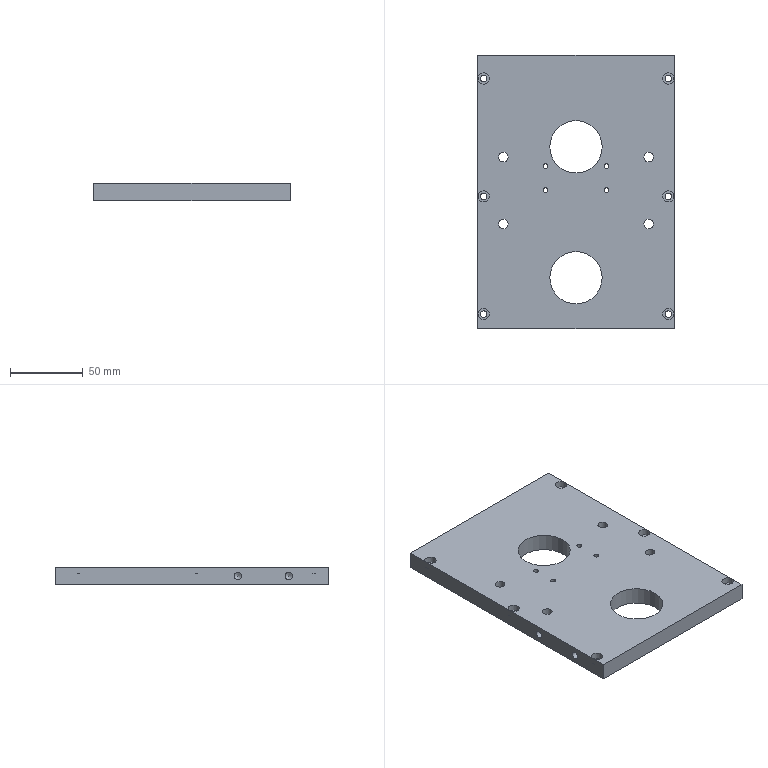Part | NX | 1 solid | 46 faces | box 135 x 188 x 12 mm | volume 273847 mm3 | cylinder 28 | plane 16 | cone 2 | commonest cylinder face diameters 4.5 x6 7.8 x6 3.3 x4 6.6 x4 11 x4 5 x2
STEP:
#1=CARTESIAN_POINT('',(-22.65,66.75,-6.));
#2=VERTEX_POINT('',#1);
#3=CARTESIAN_POINT('',(-21.,66.75,-6.));
#4=DIRECTION('',(0.,0.,-1.));
#5=DIRECTION('',(-1.,0.,0.));
#6=AXIS2_PLACEMENT_3D('',#3,#4,#5);
#7=CIRCLE('',#6,1.65);
#8=EDGE_CURVE('',#2,#2,#7,.T.);
#9=ORIENTED_EDGE('',*,*,#8,.F.);
#10=EDGE_LOOP('',(#9));
#11=FACE_BOUND('',#10,.T.);
#12=CARTESIAN_POINT('',(-22.65,50.25,-6.));
#13=VERTEX_POINT('',#12);
#14=CARTESIAN_POINT('',(-21.,50.25,-6.));
#15=DIRECTION('',(0.,0.,-1.));
#16=DIRECTION('',(-1.,0.,0.));
#17=AXIS2_PLACEMENT_3D('',#14,#15,#16);
#18=CIRCLE('',#17,1.65);
#19=EDGE_CURVE('',#13,#13,#18,.T.);
#20=ORIENTED_EDGE('',*,*,#19,.F.);
#21=EDGE_LOOP('',(#20));
#22=FACE_BOUND('',#21,.T.);
#23=CARTESIAN_POINT('',(19.35,50.25,-6.));
#24=VERTEX_POINT('',#23);
#25=CARTESIAN_POINT('',(21.,50.25,-6.));
#26=DIRECTION('',(0.,0.,-1.));
#27=DIRECTION('',(-1.,0.,0.));
#28=AXIS2_PLACEMENT_3D('',#25,#26,#27);
#29=CIRCLE('',#28,1.65);
#30=EDGE_CURVE('',#24,#24,#29,.T.);
#31=ORIENTED_EDGE('',*,*,#30,.F.);
#32=EDGE_LOOP('',(#31));
#33=FACE_BOUND('',#32,.T.);
#34=CARTESIAN_POINT('',(67.5,-45.,-6.));
#35=VERTEX_POINT('',#34);
#36=CARTESIAN_POINT('',(67.5,143.,-6.));
#37=VERTEX_POINT('',#36);
#38=CARTESIAN_POINT('',(67.5,45.,-6.));
#39=DIRECTION('',(0.,1.,0.));
#40=VECTOR('',#39,1000.);
#41=LINE('',#38,#40);
#42=EDGE_CURVE('',#35,#37,#41,.T.);
#43=ORIENTED_EDGE('',*,*,#42,.F.);
#44=CARTESIAN_POINT('',(-67.5,-45.,-6.));
#45=VERTEX_POINT('',#44);
#46=CARTESIAN_POINT('',(-67.5,-45.,-6.));
#47=DIRECTION('',(1.,0.,0.));
#48=VECTOR('',#47,1000.);
#49=LINE('',#46,#48);
#50=EDGE_CURVE('',#45,#35,#49,.T.);
#51=ORIENTED_EDGE('',*,*,#50,.F.);
#52=CARTESIAN_POINT('',(-67.5,143.,-6.));
#53=VERTEX_POINT('',#52);
#54=CARTESIAN_POINT('',(-67.5,45.,-6.));
#55=DIRECTION('',(0.,-1.,0.));
#56=VECTOR('',#55,1000.);
#57=LINE('',#54,#56);
#58=EDGE_CURVE('',#53,#45,#57,.T.);
#59=ORIENTED_EDGE('',*,*,#58,.F.);
#60=CARTESIAN_POINT('',(-67.5,143.,-6.));
#61=DIRECTION('',(1.,0.,0.));
#62=VECTOR('',#61,1000.);
#63=LINE('',#60,#62);
#64=EDGE_CURVE('',#53,#37,#63,.T.);
#65=ORIENTED_EDGE('',*,*,#64,.T.);
#66=EDGE_LOOP('',(#43,#51,#59,#65));
#67=FACE_BOUND('',#66,.T.);
#68=CARTESIAN_POINT('',(65.75,-35.,-6.));
#69=VERTEX_POINT('',#68);
#70=CARTESIAN_POINT('',(63.5,-35.,-6.));
#71=DIRECTION('',(0.,0.,1.));
#72=DIRECTION('',(1.,0.,0.));
#73=AXIS2_PLACEMENT_3D('',#70,#71,#72);
#74=CIRCLE('',#73,2.25);
#75=EDGE_CURVE('',#69,#69,#74,.T.);
#76=ORIENTED_EDGE('',*,*,#75,.T.);
#77=EDGE_LOOP('',(#76));
#78=FACE_BOUND('',#77,.T.);
#79=CARTESIAN_POINT('',(-61.25,-35.,-6.));
#80=VERTEX_POINT('',#79);
#81=CARTESIAN_POINT('',(-63.5,-35.,-6.));
#82=DIRECTION('',(0.,0.,1.));
#83=DIRECTION('',(1.,0.,0.));
#84=AXIS2_PLACEMENT_3D('',#81,#82,#83);
#85=CIRCLE('',#84,2.25);
#86=EDGE_CURVE('',#80,#80,#85,.T.);
#87=ORIENTED_EDGE('',*,*,#86,.T.);
#88=EDGE_LOOP('',(#87));
#89=FACE_BOUND('',#88,.T.);
#90=CARTESIAN_POINT('',(-61.25,127.,-6.));
#91=VERTEX_POINT('',#90);
#92=CARTESIAN_POINT('',(-63.5,127.,-6.));
#93=DIRECTION('',(0.,0.,1.));
#94=DIRECTION('',(1.,0.,0.));
#95=AXIS2_PLACEMENT_3D('',#92,#93,#94);
#96=CIRCLE('',#95,2.25);
#97=EDGE_CURVE('',#91,#91,#96,.T.);
#98=ORIENTED_EDGE('',*,*,#97,.T.);
#99=EDGE_LOOP('',(#98));
#100=FACE_BOUND('',#99,.T.);
#101=CARTESIAN_POINT('',(-61.25,46.,-6.));
#102=VERTEX_POINT('',#101);
#103=CARTESIAN_POINT('',(-63.5,46.,-6.));
#104=DIRECTION('',(0.,0.,1.));
#105=DIRECTION('',(1.,0.,0.));
#106=AXIS2_PLACEMENT_3D('',#103,#104,#105);
#107=CIRCLE('',#106,2.25);
#108=EDGE_CURVE('',#102,#102,#107,.T.);
#109=ORIENTED_EDGE('',*,*,#108,.T.);
#110=EDGE_LOOP('',(#109));
#111=FACE_BOUND('',#110,.T.);
#112=CARTESIAN_POINT('',(65.75,46.,-6.));
#113=VERTEX_POINT('',#112);
#114=CARTESIAN_POINT('',(63.5,46.,-6.));
#115=DIRECTION('',(0.,0.,1.));
#116=DIRECTION('',(1.,0.,0.));
#117=AXIS2_PLACEMENT_3D('',#114,#115,#116);
#118=CIRCLE('',#117,2.25);
#119=EDGE_CURVE('',#113,#113,#118,.T.);
#120=ORIENTED_EDGE('',*,*,#119,.T.);
#121=EDGE_LOOP('',(#120));
#122=FACE_BOUND('',#121,.T.);
#123=CARTESIAN_POINT('',(65.75,127.,-6.));
#124=VERTEX_POINT('',#123);
#125=CARTESIAN_POINT('',(63.5,127.,-6.));
#126=DIRECTION('',(0.,0.,1.));
#127=DIRECTION('',(1.,0.,0.));
#128=AXIS2_PLACEMENT_3D('',#125,#126,#127);
#129=CIRCLE('',#128,2.25);
#130=EDGE_CURVE('',#124,#124,#129,.T.);
#131=ORIENTED_EDGE('',*,*,#130,.T.);
#132=EDGE_LOOP('',(#131));
#133=FACE_BOUND('',#132,.T.);
#134=CARTESIAN_POINT('',(-55.5,73.,-6.));
#135=VERTEX_POINT('',#134);
#136=CARTESIAN_POINT('',(-50.,73.,-6.));
#137=DIRECTION('',(0.,0.,-1.));
#138=DIRECTION('',(-1.,0.,0.));
#139=AXIS2_PLACEMENT_3D('',#136,#137,#138);
#140=CIRCLE('',#139,5.5);
#141=EDGE_CURVE('',#135,#135,#140,.T.);
#142=ORIENTED_EDGE('',*,*,#141,.F.);
#143=EDGE_LOOP('',(#142));
#144=FACE_BOUND('',#143,.T.);
#145=CARTESIAN_POINT('',(-55.5,27.,-6.));
#146=VERTEX_POINT('',#145);
#147=CARTESIAN_POINT('',(-50.,27.,-6.));
#148=DIRECTION('',(0.,0.,-1.));
#149=DIRECTION('',(-1.,0.,0.));
#150=AXIS2_PLACEMENT_3D('',#147,#148,#149);
#151=CIRCLE('',#150,5.5);
#152=EDGE_CURVE('',#146,#146,#151,.T.);
#153=ORIENTED_EDGE('',*,*,#152,.F.);
#154=EDGE_LOOP('',(#153));
#155=FACE_BOUND('',#154,.T.);
#156=CARTESIAN_POINT('',(44.5,27.,-6.));
#157=VERTEX_POINT('',#156);
#158=CARTESIAN_POINT('',(50.,27.,-6.));
#159=DIRECTION('',(0.,0.,-1.));
#160=DIRECTION('',(-1.,0.,0.));
#161=AXIS2_PLACEMENT_3D('',#158,#159,#160);
#162=CIRCLE('',#161,5.5);
#163=EDGE_CURVE('',#157,#157,#162,.T.);
#164=ORIENTED_EDGE('',*,*,#163,.F.);
#165=EDGE_LOOP('',(#164));
#166=FACE_BOUND('',#165,.T.);
#167=CARTESIAN_POINT('',(44.5,73.,-6.));
#168=VERTEX_POINT('',#167);
#169=CARTESIAN_POINT('',(50.,73.,-6.));
#170=DIRECTION('',(0.,0.,-1.));
#171=DIRECTION('',(-1.,0.,0.));
#172=AXIS2_PLACEMENT_3D('',#169,#170,#171);
#173=CIRCLE('',#172,5.5);
#174=EDGE_CURVE('',#168,#168,#173,.T.);
#175=ORIENTED_EDGE('',*,*,#174,.F.);
#176=EDGE_LOOP('',(#175));
#177=FACE_BOUND('',#176,.T.);
#178=CARTESIAN_POINT('',(18.,80.,-6.));
#179=VERTEX_POINT('',#178);
#180=CARTESIAN_POINT('',(0.,80.,-6.));
#181=DIRECTION('',(0.,0.,1.));
#182=DIRECTION('',(1.,0.,0.));
#183=AXIS2_PLACEMENT_3D('',#180,#181,#182);
#184=CIRCLE('',#183,18.);
#185=EDGE_CURVE('',#179,#179,#184,.T.);
#186=ORIENTED_EDGE('',*,*,#185,.T.);
#187=EDGE_LOOP('',(#186));
#188=FACE_BOUND('',#187,.T.);
#189=CARTESIAN_POINT('',(18.,-10.,-6.));
#190=VERTEX_POINT('',#189);
#191=CARTESIAN_POINT('',(0.,-10.,-6.));
#192=DIRECTION('',(0.,0.,1.));
#193=DIRECTION('',(1.,0.,0.));
#194=AXIS2_PLACEMENT_3D('',#191,#192,#193);
#195=CIRCLE('',#194,18.);
#196=EDGE_CURVE('',#190,#190,#195,.T.);
#197=ORIENTED_EDGE('',*,*,#196,.T.);
#198=EDGE_LOOP('',(#197));
#199=FACE_BOUND('',#198,.T.);
#200=CARTESIAN_POINT('',(19.35,66.75,-6.));
#201=VERTEX_POINT('',#200);
#202=CARTESIAN_POINT('',(21.,66.75,-6.));
#203=DIRECTION('',(0.,0.,-1.));
#204=DIRECTION('',(-1.,0.,0.));
#205=AXIS2_PLACEMENT_3D('',#202,#203,#204);
#206=CIRCLE('',#205,1.65);
#207=EDGE_CURVE('',#201,#201,#206,.T.);
#208=ORIENTED_EDGE('',*,*,#207,.F.);
#209=EDGE_LOOP('',(#208));
#210=FACE_BOUND('',#209,.T.);
#211=CARTESIAN_POINT('',(0.,0.,-6.));
#212=DIRECTION('',(0.,0.,1.));
#213=DIRECTION('',(1.,0.,0.));
#214=AXIS2_PLACEMENT_3D('',#211,#212,#213);
#215=PLANE('',#214);
#216=ADVANCED_FACE('',(#11,#22,#33,#67,#78,#89,#100,#111,#122,#133,#144,#155,#166,#177,#188,#199,#210),#215,.F.);
#217=ORIENTED_EDGE('',*,*,#42,.T.);
#218=CARTESIAN_POINT('',(67.5,143.,6.));
#219=VERTEX_POINT('',#218);
#220=CARTESIAN_POINT('',(67.5,143.,172.82));
#221=DIRECTION('',(0.,0.,-1.));
#222=VECTOR('',#221,1000.);
#223=LINE('',#220,#222);
#224=EDGE_CURVE('',#219,#37,#223,.T.);
#225=ORIENTED_EDGE('',*,*,#224,.F.);
#226=CARTESIAN_POINT('',(67.5,-45.,6.));
#227=VERTEX_POINT('',#226);
#228=CARTESIAN_POINT('',(67.5,45.,6.));
#229=DIRECTION('',(0.,1.,0.));
#230=VECTOR('',#229,1000.);
#231=LINE('',#228,#230);
#232=EDGE_CURVE('',#227,#219,#231,.T.);
#233=ORIENTED_EDGE('',*,*,#232,.F.);
#234=CARTESIAN_POINT('',(67.5,-45.,6.));
#235=DIRECTION('',(0.,0.,-1.));
#236=VECTOR('',#235,1000.);
#237=LINE('',#234,#236);
#238=EDGE_CURVE('',#227,#35,#237,.T.);
#239=ORIENTED_EDGE('',*,*,#238,.T.);
#240=EDGE_LOOP('',(#217,#225,#233,#239));
#241=FACE_BOUND('',#240,.T.);
#242=CARTESIAN_POINT('',(67.5,45.,6.));
#243=DIRECTION('',(-1.,0.,0.));
#244=DIRECTION('',(0.,-1.,0.));
#245=AXIS2_PLACEMENT_3D('',#242,#243,#244);
#246=PLANE('',#245);
#247=ADVANCED_FACE('',(#241),#246,.F.);
#248=CARTESIAN_POINT('',(-67.5,17.5,2.5));
#249=VERTEX_POINT('',#248);
#250=CARTESIAN_POINT('',(-67.5,17.5,0.));
#251=DIRECTION('',(-1.,0.,0.));
#252=DIRECTION('',(0.,0.,1.));
#253=AXIS2_PLACEMENT_3D('',#250,#251,#252);
#254=CIRCLE('',#253,2.5);
#255=EDGE_CURVE('',#249,#249,#254,.T.);
#256=ORIENTED_EDGE('',*,*,#255,.F.);
#257=EDGE_LOOP('',(#256));
#258=FACE_BOUND('',#257,.T.);
#259=CARTESIAN_POINT('',(-67.5,-17.5,2.5));
#260=VERTEX_POINT('',#259);
#261=CARTESIAN_POINT('',(-67.5,-17.5,0.));
#262=DIRECTION('',(-1.,0.,0.));
#263=DIRECTION('',(0.,0.,1.));
#264=AXIS2_PLACEMENT_3D('',#261,#262,#263);
#265=CIRCLE('',#264,2.5);
#266=EDGE_CURVE('',#260,#260,#265,.T.);
#267=ORIENTED_EDGE('',*,*,#266,.F.);
#268=EDGE_LOOP('',(#267));
#269=FACE_BOUND('',#268,.T.);
#270=ORIENTED_EDGE('',*,*,#58,.T.);
#271=CARTESIAN_POINT('',(-67.5,-45.,6.));
#272=VERTEX_POINT('',#271);
#273=CARTESIAN_POINT('',(-67.5,-45.,6.));
#274=DIRECTION('',(0.,0.,-1.));
#275=VECTOR('',#274,1000.);
#276=LINE('',#273,#275);
#277=EDGE_CURVE('',#272,#45,#276,.T.);
#278=ORIENTED_EDGE('',*,*,#277,.F.);
#279=CARTESIAN_POINT('',(-67.5,143.,6.));
#280=VERTEX_POINT('',#279);
#281=CARTESIAN_POINT('',(-67.5,45.,6.));
#282=DIRECTION('',(0.,-1.,0.));
#283=VECTOR('',#282,1000.);
#284=LINE('',#281,#283);
#285=EDGE_CURVE('',#280,#272,#284,.T.);
#286=ORIENTED_EDGE('',*,*,#285,.F.);
#287=CARTESIAN_POINT('',(-67.5,143.,172.82));
#288=DIRECTION('',(0.,0.,-1.));
#289=VECTOR('',#288,1000.);
#290=LINE('',#287,#289);
#291=EDGE_CURVE('',#280,#53,#290,.T.);
#292=ORIENTED_EDGE('',*,*,#291,.T.);
#293=EDGE_LOOP('',(#270,#278,#286,#292));
#294=FACE_BOUND('',#293,.T.);
#295=CARTESIAN_POINT('',(-67.5,45.,6.));
#296=DIRECTION('',(1.,0.,0.));
#297=DIRECTION('',(0.,0.,-1.));
#298=AXIS2_PLACEMENT_3D('',#295,#296,#297);
#299=PLANE('',#298);
#300=ADVANCED_FACE('',(#258,#269,#294),#299,.F.);
#301=ORIENTED_EDGE('',*,*,#50,.T.);
#302=ORIENTED_EDGE('',*,*,#238,.F.);
#303=CARTESIAN_POINT('',(-67.5,-45.,6.));
#304=DIRECTION('',(1.,0.,0.));
#305=VECTOR('',#304,1000.);
#306=LINE('',#303,#305);
#307=EDGE_CURVE('',#272,#227,#306,.T.);
#308=ORIENTED_EDGE('',*,*,#307,.F.);
#309=ORIENTED_EDGE('',*,*,#277,.T.);
#310=EDGE_LOOP('',(#301,#302,#308,#309));
#311=FACE_BOUND('',#310,.T.);
#312=CARTESIAN_POINT('',(-67.5,-45.,6.));
#313=DIRECTION('',(0.,1.,0.));
#314=DIRECTION('',(0.,0.,1.));
#315=AXIS2_PLACEMENT_3D('',#312,#313,#314);
#316=PLANE('',#315);
#317=ADVANCED_FACE('',(#311),#316,.F.);
#318=CARTESIAN_POINT('',(-22.65,66.75,6.));
#319=VERTEX_POINT('',#318);
#320=CARTESIAN_POINT('',(-21.,66.75,6.));
#321=DIRECTION('',(0.,0.,-1.));
#322=DIRECTION('',(-1.,0.,0.));
#323=AXIS2_PLACEMENT_3D('',#320,#321,#322);
#324=CIRCLE('',#323,1.65);
#325=EDGE_CURVE('',#319,#319,#324,.T.);
#326=ORIENTED_EDGE('',*,*,#325,.T.);
#327=EDGE_LOOP('',(#326));
#328=FACE_BOUND('',#327,.T.);
#329=CARTESIAN_POINT('',(-22.65,50.25,6.));
#330=VERTEX_POINT('',#329);
#331=CARTESIAN_POINT('',(-21.,50.25,6.));
#332=DIRECTION('',(0.,0.,-1.));
#333=DIRECTION('',(-1.,0.,0.));
#334=AXIS2_PLACEMENT_3D('',#331,#332,#333);
#335=CIRCLE('',#334,1.65);
#336=EDGE_CURVE('',#330,#330,#335,.T.);
#337=ORIENTED_EDGE('',*,*,#336,.T.);
#338=EDGE_LOOP('',(#337));
#339=FACE_BOUND('',#338,.T.);
#340=CARTESIAN_POINT('',(19.35,50.25,6.));
#341=VERTEX_POINT('',#340);
#342=CARTESIAN_POINT('',(21.,50.25,6.));
#343=DIRECTION('',(0.,0.,-1.));
#344=DIRECTION('',(-1.,0.,0.));
#345=AXIS2_PLACEMENT_3D('',#342,#343,#344);
#346=CIRCLE('',#345,1.65);
#347=EDGE_CURVE('',#341,#341,#346,.T.);
#348=ORIENTED_EDGE('',*,*,#347,.T.);
#349=EDGE_LOOP('',(#348));
#350=FACE_BOUND('',#349,.T.);
#351=CARTESIAN_POINT('',(19.35,66.75,6.));
#352=VERTEX_POINT('',#351);
#353=CARTESIAN_POINT('',(21.,66.75,6.));
#354=DIRECTION('',(0.,0.,-1.));
#355=DIRECTION('',(-1.,0.,0.));
#356=AXIS2_PLACEMENT_3D('',#353,#354,#355);
#357=CIRCLE('',#356,1.65);
#358=EDGE_CURVE('',#352,#352,#357,.T.);
#359=ORIENTED_EDGE('',*,*,#358,.T.);
#360=EDGE_LOOP('',(#359));
#361=FACE_BOUND('',#360,.T.);
#362=CARTESIAN_POINT('',(18.,-10.,6.));
#363=VERTEX_POINT('',#362);
#364=CARTESIAN_POINT('',(0.,-10.,6.));
#365=DIRECTION('',(0.,0.,1.));
#366=DIRECTION('',(1.,0.,0.));
#367=AXIS2_PLACEMENT_3D('',#364,#365,#366);
#368=CIRCLE('',#367,18.);
#369=EDGE_CURVE('',#363,#363,#368,.T.);
#370=ORIENTED_EDGE('',*,*,#369,.F.);
#371=EDGE_LOOP('',(#370));
#372=FACE_BOUND('',#371,.T.);
#373=CARTESIAN_POINT('',(18.,80.,6.));
#374=VERTEX_POINT('',#373);
#375=CARTESIAN_POINT('',(0.,80.,6.));
#376=DIRECTION('',(0.,0.,1.));
#377=DIRECTION('',(1.,0.,0.));
#378=AXIS2_PLACEMENT_3D('',#375,#376,#377);
#379=CIRCLE('',#378,18.);
#380=EDGE_CURVE('',#374,#374,#379,.T.);
#381=ORIENTED_EDGE('',*,*,#380,.F.);
#382=EDGE_LOOP('',(#381));
#383=FACE_BOUND('',#382,.T.);
#384=CARTESIAN_POINT('',(46.7,73.,6.));
#385=VERTEX_POINT('',#384);
#386=CARTESIAN_POINT('',(50.,73.,6.));
#387=DIRECTION('',(0.,0.,-1.));
#388=DIRECTION('',(-1.,0.,0.));
#389=AXIS2_PLACEMENT_3D('',#386,#387,#388);
#390=CIRCLE('',#389,3.3);
#391=EDGE_CURVE('',#385,#385,#390,.T.);
#392=ORIENTED_EDGE('',*,*,#391,.T.);
#393=EDGE_LOOP('',(#392));
#394=FACE_BOUND('',#393,.T.);
#395=CARTESIAN_POINT('',(46.7,27.,6.));
#396=VERTEX_POINT('',#395);
#397=CARTESIAN_POINT('',(50.,27.,6.));
#398=DIRECTION('',(0.,0.,-1.));
#399=DIRECTION('',(-1.,0.,0.));
#400=AXIS2_PLACEMENT_3D('',#397,#398,#399);
#401=CIRCLE('',#400,3.3);
#402=EDGE_CURVE('',#396,#396,#401,.T.);
#403=ORIENTED_EDGE('',*,*,#402,.T.);
#404=EDGE_LOOP('',(#403));
#405=FACE_BOUND('',#404,.T.);
#406=CARTESIAN_POINT('',(-53.3,27.,6.));
#407=VERTEX_POINT('',#406);
#408=CARTESIAN_POINT('',(-50.,27.,6.));
#409=DIRECTION('',(0.,0.,-1.));
#410=DIRECTION('',(-1.,0.,0.));
#411=AXIS2_PLACEMENT_3D('',#408,#409,#410);
#412=CIRCLE('',#411,3.3);
#413=EDGE_CURVE('',#407,#407,#412,.T.);
#414=ORIENTED_EDGE('',*,*,#413,.T.);
#415=EDGE_LOOP('',(#414));
#416=FACE_BOUND('',#415,.T.);
#417=CARTESIAN_POINT('',(-53.3,73.,6.));
#418=VERTEX_POINT('',#417);
#419=CARTESIAN_POINT('',(-50.,73.,6.));
#420=DIRECTION('',(0.,0.,-1.));
#421=DIRECTION('',(-1.,0.,0.));
#422=AXIS2_PLACEMENT_3D('',#419,#420,#421);
#423=CIRCLE('',#422,3.3);
#424=EDGE_CURVE('',#418,#418,#423,.T.);
#425=ORIENTED_EDGE('',*,*,#424,.T.);
#426=EDGE_LOOP('',(#425));
#427=FACE_BOUND('',#426,.T.);
#428=CARTESIAN_POINT('',(67.4,127.,6.));
#429=VERTEX_POINT('',#428);
#430=CARTESIAN_POINT('',(63.5,127.,6.));
#431=DIRECTION('',(0.,0.,1.));
#432=DIRECTION('',(1.,0.,0.));
#433=AXIS2_PLACEMENT_3D('',#430,#431,#432);
#434=CIRCLE('',#433,3.9);
#435=EDGE_CURVE('',#429,#429,#434,.T.);
#436=ORIENTED_EDGE('',*,*,#435,.F.);
#437=EDGE_LOOP('',(#436));
#438=FACE_BOUND('',#437,.T.);
#439=CARTESIAN_POINT('',(67.4,46.,6.));
#440=VERTEX_POINT('',#439);
#441=CARTESIAN_POINT('',(63.5,46.,6.));
#442=DIRECTION('',(0.,0.,1.));
#443=DIRECTION('',(1.,0.,0.));
#444=AXIS2_PLACEMENT_3D('',#441,#442,#443);
#445=CIRCLE('',#444,3.9);
#446=EDGE_CURVE('',#440,#440,#445,.T.);
#447=ORIENTED_EDGE('',*,*,#446,.F.);
#448=EDGE_LOOP('',(#447));
#449=FACE_BOUND('',#448,.T.);
#450=CARTESIAN_POINT('',(-59.6,46.,6.));
#451=VERTEX_POINT('',#450);
#452=CARTESIAN_POINT('',(-63.5,46.,6.));
#453=DIRECTION('',(0.,0.,1.));
#454=DIRECTION('',(1.,0.,0.));
#455=AXIS2_PLACEMENT_3D('',#452,#453,#454);
#456=CIRCLE('',#455,3.9);
#457=EDGE_CURVE('',#451,#451,#456,.T.);
#458=ORIENTED_EDGE('',*,*,#457,.F.);
#459=EDGE_LOOP('',(#458));
#460=FACE_BOUND('',#459,.T.);
#461=CARTESIAN_POINT('',(-59.6,127.,6.));
#462=VERTEX_POINT('',#461);
#463=CARTESIAN_POINT('',(-63.5,127.,6.));
#464=DIRECTION('',(0.,0.,1.));
#465=DIRECTION('',(1.,0.,0.));
#466=AXIS2_PLACEMENT_3D('',#463,#464,#465);
#467=CIRCLE('',#466,3.9);
#468=EDGE_CURVE('',#462,#462,#467,.T.);
#469=ORIENTED_EDGE('',*,*,#468,.F.);
#470=EDGE_LOOP('',(#469));
#471=FACE_BOUND('',#470,.T.);
#472=CARTESIAN_POINT('',(-59.6,-35.,6.));
#473=VERTEX_POINT('',#472);
#474=CARTESIAN_POINT('',(-63.5,-35.,6.));
#475=DIRECTION('',(0.,0.,1.));
#476=DIRECTION('',(1.,0.,0.));
#477=AXIS2_PLACEMENT_3D('',#474,#475,#476);
#478=CIRCLE('',#477,3.9);
#479=EDGE_CURVE('',#473,#473,#478,.T.);
#480=ORIENTED_EDGE('',*,*,#479,.F.);
#481=EDGE_LOOP('',(#480));
#482=FACE_BOUND('',#481,.T.);
#483=CARTESIAN_POINT('',(67.4,-35.,6.));
#484=VERTEX_POINT('',#483);
#485=CARTESIAN_POINT('',(63.5,-35.,6.));
#486=DIRECTION('',(0.,0.,1.));
#487=DIRECTION('',(1.,0.,0.));
#488=AXIS2_PLACEMENT_3D('',#485,#486,#487);
#489=CIRCLE('',#488,3.9);
#490=EDGE_CURVE('',#484,#484,#489,.T.);
#491=ORIENTED_EDGE('',*,*,#490,.F.);
#492=EDGE_LOOP('',(#491));
#493=FACE_BOUND('',#492,.T.);
#494=ORIENTED_EDGE('',*,*,#232,.T.);
#495=CARTESIAN_POINT('',(-67.5,143.,6.));
#496=DIRECTION('',(1.,0.,0.));
#497=VECTOR('',#496,1000.);
#498=LINE('',#495,#497);
#499=EDGE_CURVE('',#280,#219,#498,.T.);
#500=ORIENTED_EDGE('',*,*,#499,.F.);
#501=ORIENTED_EDGE('',*,*,#285,.T.);
#502=ORIENTED_EDGE('',*,*,#307,.T.);
#503=EDGE_LOOP('',(#494,#500,#501,#502));
#504=FACE_BOUND('',#503,.T.);
#505=CARTESIAN_POINT('',(0.,0.,6.));
#506=DIRECTION('',(0.,0.,1.));
#507=DIRECTION('',(1.,0.,0.));
#508=AXIS2_PLACEMENT_3D('',#505,#506,#507);
#509=PLANE('',#508);
#510=ADVANCED_FACE('',(#328,#339,#350,#361,#372,#383,#394,#405,#416,#427,#438,#449,#460,#471,#482,#493,#504),#509,.T.);
#511=ORIENTED_EDGE('',*,*,#291,.F.);
#512=ORIENTED_EDGE('',*,*,#499,.T.);
#513=ORIENTED_EDGE('',*,*,#224,.T.);
#514=ORIENTED_EDGE('',*,*,#64,.F.);
#515=EDGE_LOOP('',(#511,#512,#513,#514));
#516=FACE_BOUND('',#515,.T.);
#517=CARTESIAN_POINT('',(-67.5,143.,172.82));
#518=DIRECTION('',(0.,1.,0.));
#519=DIRECTION('',(0.,0.,1.));
#520=AXIS2_PLACEMENT_3D('',#517,#518,#519);
#521=PLANE('',#520);
#522=ADVANCED_FACE('',(#516),#521,.T.);
#523=ORIENTED_EDGE('',*,*,#75,.F.);
#524=EDGE_LOOP('',(#523));
#525=FACE_BOUND('',#524,.T.);
#526=CARTESIAN_POINT('',(65.75,-35.,1.6));
#527=VERTEX_POINT('',#526);
#528=CARTESIAN_POINT('',(63.5,-35.,1.6));
#529=DIRECTION('',(0.,0.,1.));
#530=DIRECTION('',(1.,0.,0.));
#531=AXIS2_PLACEMENT_3D('',#528,#529,#530);
#532=CIRCLE('',#531,2.25);
#533=EDGE_CURVE('',#527,#527,#532,.T.);
#534=ORIENTED_EDGE('',*,*,#533,.T.);
#535=EDGE_LOOP('',(#534));
#536=FACE_BOUND('',#535,.T.);
#537=CARTESIAN_POINT('',(63.5,-35.,6.));
#538=DIRECTION('',(0.,0.,1.));
#539=DIRECTION('',(1.,0.,0.));
#540=AXIS2_PLACEMENT_3D('',#537,#538,#539);
#541=CYLINDRICAL_SURFACE('',#540,2.25);
#542=ADVANCED_FACE('',(#525,#536),#541,.F.);
#543=ORIENTED_EDGE('',*,*,#533,.F.);
#544=EDGE_LOOP('',(#543));
#545=FACE_BOUND('',#544,.T.);
#546=CARTESIAN_POINT('',(67.4,-35.,1.6));
#547=VERTEX_POINT('',#546);
#548=CARTESIAN_POINT('',(63.5,-35.,1.6));
#549=DIRECTION('',(0.,0.,1.));
#550=DIRECTION('',(1.,0.,0.));
#551=AXIS2_PLACEMENT_3D('',#548,#549,#550);
#552=CIRCLE('',#551,3.9);
#553=EDGE_CURVE('',#547,#547,#552,.T.);
#554=ORIENTED_EDGE('',*,*,#553,.T.);
#555=EDGE_LOOP('',(#554));
#556=FACE_BOUND('',#555,.T.);
#557=CARTESIAN_POINT('',(65.75,-35.,1.6));
#558=DIRECTION('',(0.,0.,-1.));
#559=DIRECTION('',(-1.,0.,0.));
#560=AXIS2_PLACEMENT_3D('',#557,#558,#559);
#561=PLANE('',#560);
#562=ADVANCED_FACE('',(#545,#556),#561,.F.);
#563=ORIENTED_EDGE('',*,*,#553,.F.);
#564=EDGE_LOOP('',(#563));
#565=FACE_BOUND('',#564,.T.);
#566=ORIENTED_EDGE('',*,*,#490,.T.);
#567=EDGE_LOOP('',(#566));
#568=FACE_BOUND('',#567,.T.);
#569=CARTESIAN_POINT('',(63.5,-35.,6.));
#570=DIRECTION('',(0.,0.,1.));
#571=DIRECTION('',(1.,0.,0.));
#572=AXIS2_PLACEMENT_3D('',#569,#570,#571);
#573=CYLINDRICAL_SURFACE('',#572,3.9);
#574=ADVANCED_FACE('',(#565,#568),#573,.F.);
#575=ORIENTED_EDGE('',*,*,#86,.F.);
#576=EDGE_LOOP('',(#575));
#577=FACE_BOUND('',#576,.T.);
#578=CARTESIAN_POINT('',(-61.25,-35.,1.6));
#579=VERTEX_POINT('',#578);
#580=CARTESIAN_POINT('',(-63.5,-35.,1.6));
#581=DIRECTION('',(0.,0.,1.));
#582=DIRECTION('',(1.,0.,0.));
#583=AXIS2_PLACEMENT_3D('',#580,#581,#582);
#584=CIRCLE('',#583,2.25);
#585=EDGE_CURVE('',#579,#579,#584,.T.);
#586=ORIENTED_EDGE('',*,*,#585,.T.);
#587=EDGE_LOOP('',(#586));
#588=FACE_BOUND('',#587,.T.);
#589=CARTESIAN_POINT('',(-63.5,-35.,6.));
#590=DIRECTION('',(0.,0.,1.));
#591=DIRECTION('',(1.,0.,0.));
#592=AXIS2_PLACEMENT_3D('',#589,#590,#591);
#593=CYLINDRICAL_SURFACE('',#592,2.25);
#594=ADVANCED_FACE('',(#577,#588),#593,.F.);
#595=ORIENTED_EDGE('',*,*,#585,.F.);
#596=EDGE_LOOP('',(#595));
#597=FACE_BOUND('',#596,.T.);
#598=CARTESIAN_POINT('',(-59.6,-35.,1.6));
#599=VERTEX_POINT('',#598);
#600=CARTESIAN_POINT('',(-63.5,-35.,1.6));
#601=DIRECTION('',(0.,0.,1.));
#602=DIRECTION('',(1.,0.,0.));
#603=AXIS2_PLACEMENT_3D('',#600,#601,#602);
#604=CIRCLE('',#603,3.9);
#605=EDGE_CURVE('',#599,#599,#604,.T.);
#606=ORIENTED_EDGE('',*,*,#605,.T.);
#607=EDGE_LOOP('',(#606));
#608=FACE_BOUND('',#607,.T.);
#609=CARTESIAN_POINT('',(-61.25,-35.,1.6));
#610=DIRECTION('',(0.,0.,-1.));
#611=DIRECTION('',(-1.,0.,0.));
#612=AXIS2_PLACEMENT_3D('',#609,#610,#611);
#613=PLANE('',#612);
#614=ADVANCED_FACE('',(#597,#608),#613,.F.);
#615=ORIENTED_EDGE('',*,*,#605,.F.);
#616=EDGE_LOOP('',(#615));
#617=FACE_BOUND('',#616,.T.);
#618=ORIENTED_EDGE('',*,*,#479,.T.);
#619=EDGE_LOOP('',(#618));
#620=FACE_BOUND('',#619,.T.);
#621=CARTESIAN_POINT('',(-63.5,-35.,6.));
#622=DIRECTION('',(0.,0.,1.));
#623=DIRECTION('',(1.,0.,0.));
#624=AXIS2_PLACEMENT_3D('',#621,#622,#623);
#625=CYLINDRICAL_SURFACE('',#624,3.9);
#626=ADVANCED_FACE('',(#617,#620),#625,.F.);
#627=ORIENTED_EDGE('',*,*,#97,.F.);
#628=EDGE_LOOP('',(#627));
#629=FACE_BOUND('',#628,.T.);
#630=CARTESIAN_POINT('',(-61.25,127.,1.6));
#631=VERTEX_POINT('',#630);
#632=CARTESIAN_POINT('',(-63.5,127.,1.6));
#633=DIRECTION('',(0.,0.,1.));
#634=DIRECTION('',(1.,0.,0.));
#635=AXIS2_PLACEMENT_3D('',#632,#633,#634);
#636=CIRCLE('',#635,2.25);
#637=EDGE_CURVE('',#631,#631,#636,.T.);
#638=ORIENTED_EDGE('',*,*,#637,.T.);
#639=EDGE_LOOP('',(#638));
#640=FACE_BOUND('',#639,.T.);
#641=CARTESIAN_POINT('',(-63.5,127.,6.));
#642=DIRECTION('',(0.,0.,1.));
#643=DIRECTION('',(1.,0.,0.));
#644=AXIS2_PLACEMENT_3D('',#641,#642,#643);
#645=CYLINDRICAL_SURFACE('',#644,2.25);
#646=ADVANCED_FACE('',(#629,#640),#645,.F.);
#647=ORIENTED_EDGE('',*,*,#637,.F.);
#648=EDGE_LOOP('',(#647));
#649=FACE_BOUND('',#648,.T.);
#650=CARTESIAN_POINT('',(-59.6,127.,1.6));
#651=VERTEX_POINT('',#650);
#652=CARTESIAN_POINT('',(-63.5,127.,1.6));
#653=DIRECTION('',(0.,0.,1.));
#654=DIRECTION('',(1.,0.,0.));
#655=AXIS2_PLACEMENT_3D('',#652,#653,#654);
#656=CIRCLE('',#655,3.9);
#657=EDGE_CURVE('',#651,#651,#656,.T.);
#658=ORIENTED_EDGE('',*,*,#657,.T.);
#659=EDGE_LOOP('',(#658));
#660=FACE_BOUND('',#659,.T.);
#661=CARTESIAN_POINT('',(-61.25,127.,1.6));
#662=DIRECTION('',(0.,0.,-1.));
#663=DIRECTION('',(-1.,0.,0.));
#664=AXIS2_PLACEMENT_3D('',#661,#662,#663);
#665=PLANE('',#664);
#666=ADVANCED_FACE('',(#649,#660),#665,.F.);
#667=ORIENTED_EDGE('',*,*,#657,.F.);
#668=EDGE_LOOP('',(#667));
#669=FACE_BOUND('',#668,.T.);
#670=ORIENTED_EDGE('',*,*,#468,.T.);
#671=EDGE_LOOP('',(#670));
#672=FACE_BOUND('',#671,.T.);
#673=CARTESIAN_POINT('',(-63.5,127.,6.));
#674=DIRECTION('',(0.,0.,1.));
#675=DIRECTION('',(1.,0.,0.));
#676=AXIS2_PLACEMENT_3D('',#673,#674,#675);
#677=CYLINDRICAL_SURFACE('',#676,3.9);
#678=ADVANCED_FACE('',(#669,#672),#677,.F.);
#679=ORIENTED_EDGE('',*,*,#108,.F.);
#680=EDGE_LOOP('',(#679));
#681=FACE_BOUND('',#680,.T.);
#682=CARTESIAN_POINT('',(-61.25,46.,1.6));
#683=VERTEX_POINT('',#682);
#684=CARTESIAN_POINT('',(-63.5,46.,1.6));
#685=DIRECTION('',(0.,0.,1.));
#686=DIRECTION('',(1.,0.,0.));
#687=AXIS2_PLACEMENT_3D('',#684,#685,#686);
#688=CIRCLE('',#687,2.25);
#689=EDGE_CURVE('',#683,#683,#688,.T.);
#690=ORIENTED_EDGE('',*,*,#689,.T.);
#691=EDGE_LOOP('',(#690));
#692=FACE_BOUND('',#691,.T.);
#693=CARTESIAN_POINT('',(-63.5,46.,6.));
#694=DIRECTION('',(0.,0.,1.));
#695=DIRECTION('',(1.,0.,0.));
#696=AXIS2_PLACEMENT_3D('',#693,#694,#695);
#697=CYLINDRICAL_SURFACE('',#696,2.25);
#698=ADVANCED_FACE('',(#681,#692),#697,.F.);
#699=ORIENTED_EDGE('',*,*,#689,.F.);
#700=EDGE_LOOP('',(#699));
#701=FACE_BOUND('',#700,.T.);
#702=CARTESIAN_POINT('',(-59.6,46.,1.6));
#703=VERTEX_POINT('',#702);
#704=CARTESIAN_POINT('',(-63.5,46.,1.6));
#705=DIRECTION('',(0.,0.,1.));
#706=DIRECTION('',(1.,0.,0.));
#707=AXIS2_PLACEMENT_3D('',#704,#705,#706);
#708=CIRCLE('',#707,3.9);
#709=EDGE_CURVE('',#703,#703,#708,.T.);
#710=ORIENTED_EDGE('',*,*,#709,.T.);
#711=EDGE_LOOP('',(#710));
#712=FACE_BOUND('',#711,.T.);
#713=CARTESIAN_POINT('',(-61.25,46.,1.6));
#714=DIRECTION('',(0.,0.,-1.));
#715=DIRECTION('',(-1.,0.,0.));
#716=AXIS2_PLACEMENT_3D('',#713,#714,#715);
#717=PLANE('',#716);
#718=ADVANCED_FACE('',(#701,#712),#717,.F.);
#719=ORIENTED_EDGE('',*,*,#709,.F.);
#720=EDGE_LOOP('',(#719));
#721=FACE_BOUND('',#720,.T.);
#722=ORIENTED_EDGE('',*,*,#457,.T.);
#723=EDGE_LOOP('',(#722));
#724=FACE_BOUND('',#723,.T.);
#725=CARTESIAN_POINT('',(-63.5,46.,6.));
#726=DIRECTION('',(0.,0.,1.));
#727=DIRECTION('',(1.,0.,0.));
#728=AXIS2_PLACEMENT_3D('',#725,#726,#727);
#729=CYLINDRICAL_SURFACE('',#728,3.9);
#730=ADVANCED_FACE('',(#721,#724),#729,.F.);
#731=ORIENTED_EDGE('',*,*,#119,.F.);
#732=EDGE_LOOP('',(#731));
#733=FACE_BOUND('',#732,.T.);
#734=CARTESIAN_POINT('',(65.75,46.,1.6));
#735=VERTEX_POINT('',#734);
#736=CARTESIAN_POINT('',(63.5,46.,1.6));
#737=DIRECTION('',(0.,0.,1.));
#738=DIRECTION('',(1.,0.,0.));
#739=AXIS2_PLACEMENT_3D('',#736,#737,#738);
#740=CIRCLE('',#739,2.25);
#741=EDGE_CURVE('',#735,#735,#740,.T.);
#742=ORIENTED_EDGE('',*,*,#741,.T.);
#743=EDGE_LOOP('',(#742));
#744=FACE_BOUND('',#743,.T.);
#745=CARTESIAN_POINT('',(63.5,46.,6.));
#746=DIRECTION('',(0.,0.,1.));
#747=DIRECTION('',(1.,0.,0.));
#748=AXIS2_PLACEMENT_3D('',#745,#746,#747);
#749=CYLINDRICAL_SURFACE('',#748,2.25);
#750=ADVANCED_FACE('',(#733,#744),#749,.F.);
#751=ORIENTED_EDGE('',*,*,#741,.F.);
#752=EDGE_LOOP('',(#751));
#753=FACE_BOUND('',#752,.T.);
#754=CARTESIAN_POINT('',(67.4,46.,1.6));
#755=VERTEX_POINT('',#754);
#756=CARTESIAN_POINT('',(63.5,46.,1.6));
#757=DIRECTION('',(0.,0.,1.));
#758=DIRECTION('',(1.,0.,0.));
#759=AXIS2_PLACEMENT_3D('',#756,#757,#758);
#760=CIRCLE('',#759,3.9);
#761=EDGE_CURVE('',#755,#755,#760,.T.);
#762=ORIENTED_EDGE('',*,*,#761,.T.);
#763=EDGE_LOOP('',(#762));
#764=FACE_BOUND('',#763,.T.);
#765=CARTESIAN_POINT('',(65.75,46.,1.6));
#766=DIRECTION('',(0.,0.,-1.));
#767=DIRECTION('',(-1.,0.,0.));
#768=AXIS2_PLACEMENT_3D('',#765,#766,#767);
#769=PLANE('',#768);
#770=ADVANCED_FACE('',(#753,#764),#769,.F.);
#771=ORIENTED_EDGE('',*,*,#761,.F.);
#772=EDGE_LOOP('',(#771));
#773=FACE_BOUND('',#772,.T.);
#774=ORIENTED_EDGE('',*,*,#446,.T.);
#775=EDGE_LOOP('',(#774));
#776=FACE_BOUND('',#775,.T.);
#777=CARTESIAN_POINT('',(63.5,46.,6.));
#778=DIRECTION('',(0.,0.,1.));
#779=DIRECTION('',(1.,0.,0.));
#780=AXIS2_PLACEMENT_3D('',#777,#778,#779);
#781=CYLINDRICAL_SURFACE('',#780,3.9);
#782=ADVANCED_FACE('',(#773,#776),#781,.F.);
#783=ORIENTED_EDGE('',*,*,#130,.F.);
#784=EDGE_LOOP('',(#783));
#785=FACE_BOUND('',#784,.T.);
#786=CARTESIAN_POINT('',(65.75,127.,1.6));
#787=VERTEX_POINT('',#786);
#788=CARTESIAN_POINT('',(63.5,127.,1.6));
#789=DIRECTION('',(0.,0.,1.));
#790=DIRECTION('',(1.,0.,0.));
#791=AXIS2_PLACEMENT_3D('',#788,#789,#790);
#792=CIRCLE('',#791,2.25);
#793=EDGE_CURVE('',#787,#787,#792,.T.);
#794=ORIENTED_EDGE('',*,*,#793,.T.);
#795=EDGE_LOOP('',(#794));
#796=FACE_BOUND('',#795,.T.);
#797=CARTESIAN_POINT('',(63.5,127.,6.));
#798=DIRECTION('',(0.,0.,1.));
#799=DIRECTION('',(1.,0.,0.));
#800=AXIS2_PLACEMENT_3D('',#797,#798,#799);
#801=CYLINDRICAL_SURFACE('',#800,2.25);
#802=ADVANCED_FACE('',(#785,#796),#801,.F.);
#803=ORIENTED_EDGE('',*,*,#793,.F.);
#804=EDGE_LOOP('',(#803));
#805=FACE_BOUND('',#804,.T.);
#806=CARTESIAN_POINT('',(67.4,127.,1.6));
#807=VERTEX_POINT('',#806);
#808=CARTESIAN_POINT('',(63.5,127.,1.6));
#809=DIRECTION('',(0.,0.,1.));
#810=DIRECTION('',(1.,0.,0.));
#811=AXIS2_PLACEMENT_3D('',#808,#809,#810);
#812=CIRCLE('',#811,3.9);
#813=EDGE_CURVE('',#807,#807,#812,.T.);
#814=ORIENTED_EDGE('',*,*,#813,.T.);
#815=EDGE_LOOP('',(#814));
#816=FACE_BOUND('',#815,.T.);
#817=CARTESIAN_POINT('',(65.75,127.,1.6));
#818=DIRECTION('',(0.,0.,-1.));
#819=DIRECTION('',(-1.,0.,0.));
#820=AXIS2_PLACEMENT_3D('',#817,#818,#819);
#821=PLANE('',#820);
#822=ADVANCED_FACE('',(#805,#816),#821,.F.);
#823=ORIENTED_EDGE('',*,*,#813,.F.);
#824=EDGE_LOOP('',(#823));
#825=FACE_BOUND('',#824,.T.);
#826=ORIENTED_EDGE('',*,*,#435,.T.);
#827=EDGE_LOOP('',(#826));
#828=FACE_BOUND('',#827,.T.);
#829=CARTESIAN_POINT('',(63.5,127.,6.));
#830=DIRECTION('',(0.,0.,1.));
#831=DIRECTION('',(1.,0.,0.));
#832=AXIS2_PLACEMENT_3D('',#829,#830,#831);
#833=CYLINDRICAL_SURFACE('',#832,3.9);
#834=ADVANCED_FACE('',(#825,#828),#833,.F.);
#835=ORIENTED_EDGE('',*,*,#424,.F.);
#836=EDGE_LOOP('',(#835));
#837=FACE_BOUND('',#836,.T.);
#838=CARTESIAN_POINT('',(-53.3,73.,0.4));
#839=VERTEX_POINT('',#838);
#840=CARTESIAN_POINT('',(-50.,73.,0.4));
#841=DIRECTION('',(0.,0.,-1.));
#842=DIRECTION('',(-1.,0.,0.));
#843=AXIS2_PLACEMENT_3D('',#840,#841,#842);
#844=CIRCLE('',#843,3.3);
#845=EDGE_CURVE('',#839,#839,#844,.T.);
#846=ORIENTED_EDGE('',*,*,#845,.T.);
#847=EDGE_LOOP('',(#846));
#848=FACE_BOUND('',#847,.T.);
#849=CARTESIAN_POINT('',(-50.,73.,-6.));
#850=DIRECTION('',(0.,0.,-1.));
#851=DIRECTION('',(-1.,0.,0.));
#852=AXIS2_PLACEMENT_3D('',#849,#850,#851);
#853=CYLINDRICAL_SURFACE('',#852,3.3);
#854=ADVANCED_FACE('',(#837,#848),#853,.F.);
#855=ORIENTED_EDGE('',*,*,#845,.F.);
#856=EDGE_LOOP('',(#855));
#857=FACE_BOUND('',#856,.T.);
#858=CARTESIAN_POINT('',(-55.5,73.,0.4));
#859=VERTEX_POINT('',#858);
#860=CARTESIAN_POINT('',(-50.,73.,0.4));
#861=DIRECTION('',(0.,0.,-1.));
#862=DIRECTION('',(-1.,0.,0.));
#863=AXIS2_PLACEMENT_3D('',#860,#861,#862);
#864=CIRCLE('',#863,5.5);
#865=EDGE_CURVE('',#859,#859,#864,.T.);
#866=ORIENTED_EDGE('',*,*,#865,.T.);
#867=EDGE_LOOP('',(#866));
#868=FACE_BOUND('',#867,.T.);
#869=CARTESIAN_POINT('',(-46.7,73.,0.4));
#870=DIRECTION('',(0.,0.,1.));
#871=DIRECTION('',(1.,0.,0.));
#872=AXIS2_PLACEMENT_3D('',#869,#870,#871);
#873=PLANE('',#872);
#874=ADVANCED_FACE('',(#857,#868),#873,.F.);
#875=ORIENTED_EDGE('',*,*,#865,.F.);
#876=EDGE_LOOP('',(#875));
#877=FACE_BOUND('',#876,.T.);
#878=ORIENTED_EDGE('',*,*,#141,.T.);
#879=EDGE_LOOP('',(#878));
#880=FACE_BOUND('',#879,.T.);
#881=CARTESIAN_POINT('',(-50.,73.,-6.));
#882=DIRECTION('',(0.,0.,-1.));
#883=DIRECTION('',(-1.,0.,0.));
#884=AXIS2_PLACEMENT_3D('',#881,#882,#883);
#885=CYLINDRICAL_SURFACE('',#884,5.5);
#886=ADVANCED_FACE('',(#877,#880),#885,.F.);
#887=ORIENTED_EDGE('',*,*,#413,.F.);
#888=EDGE_LOOP('',(#887));
#889=FACE_BOUND('',#888,.T.);
#890=CARTESIAN_POINT('',(-53.3,27.,0.4));
#891=VERTEX_POINT('',#890);
#892=CARTESIAN_POINT('',(-50.,27.,0.4));
#893=DIRECTION('',(0.,0.,-1.));
#894=DIRECTION('',(-1.,0.,0.));
#895=AXIS2_PLACEMENT_3D('',#892,#893,#894);
#896=CIRCLE('',#895,3.3);
#897=EDGE_CURVE('',#891,#891,#896,.T.);
#898=ORIENTED_EDGE('',*,*,#897,.T.);
#899=EDGE_LOOP('',(#898));
#900=FACE_BOUND('',#899,.T.);
#901=CARTESIAN_POINT('',(-50.,27.,-6.));
#902=DIRECTION('',(0.,0.,-1.));
#903=DIRECTION('',(-1.,0.,0.));
#904=AXIS2_PLACEMENT_3D('',#901,#902,#903);
#905=CYLINDRICAL_SURFACE('',#904,3.3);
#906=ADVANCED_FACE('',(#889,#900),#905,.F.);
#907=ORIENTED_EDGE('',*,*,#897,.F.);
#908=EDGE_LOOP('',(#907));
#909=FACE_BOUND('',#908,.T.);
#910=CARTESIAN_POINT('',(-55.5,27.,0.4));
#911=VERTEX_POINT('',#910);
#912=CARTESIAN_POINT('',(-50.,27.,0.4));
#913=DIRECTION('',(0.,0.,-1.));
#914=DIRECTION('',(-1.,0.,0.));
#915=AXIS2_PLACEMENT_3D('',#912,#913,#914);
#916=CIRCLE('',#915,5.5);
#917=EDGE_CURVE('',#911,#911,#916,.T.);
#918=ORIENTED_EDGE('',*,*,#917,.T.);
#919=EDGE_LOOP('',(#918));
#920=FACE_BOUND('',#919,.T.);
#921=CARTESIAN_POINT('',(-46.7,27.,0.4));
#922=DIRECTION('',(0.,0.,1.));
#923=DIRECTION('',(1.,0.,0.));
#924=AXIS2_PLACEMENT_3D('',#921,#922,#923);
#925=PLANE('',#924);
#926=ADVANCED_FACE('',(#909,#920),#925,.F.);
#927=ORIENTED_EDGE('',*,*,#917,.F.);
#928=EDGE_LOOP('',(#927));
#929=FACE_BOUND('',#928,.T.);
#930=ORIENTED_EDGE('',*,*,#152,.T.);
#931=EDGE_LOOP('',(#930));
#932=FACE_BOUND('',#931,.T.);
#933=CARTESIAN_POINT('',(-50.,27.,-6.));
#934=DIRECTION('',(0.,0.,-1.));
#935=DIRECTION('',(-1.,0.,0.));
#936=AXIS2_PLACEMENT_3D('',#933,#934,#935);
#937=CYLINDRICAL_SURFACE('',#936,5.5);
#938=ADVANCED_FACE('',(#929,#932),#937,.F.);
#939=ORIENTED_EDGE('',*,*,#402,.F.);
#940=EDGE_LOOP('',(#939));
#941=FACE_BOUND('',#940,.T.);
#942=CARTESIAN_POINT('',(46.7,27.,0.4));
#943=VERTEX_POINT('',#942);
#944=CARTESIAN_POINT('',(50.,27.,0.4));
#945=DIRECTION('',(0.,0.,-1.));
#946=DIRECTION('',(-1.,0.,0.));
#947=AXIS2_PLACEMENT_3D('',#944,#945,#946);
#948=CIRCLE('',#947,3.3);
#949=EDGE_CURVE('',#943,#943,#948,.T.);
#950=ORIENTED_EDGE('',*,*,#949,.T.);
#951=EDGE_LOOP('',(#950));
#952=FACE_BOUND('',#951,.T.);
#953=CARTESIAN_POINT('',(50.,27.,-6.));
#954=DIRECTION('',(0.,0.,-1.));
#955=DIRECTION('',(-1.,0.,0.));
#956=AXIS2_PLACEMENT_3D('',#953,#954,#955);
#957=CYLINDRICAL_SURFACE('',#956,3.3);
#958=ADVANCED_FACE('',(#941,#952),#957,.F.);
#959=ORIENTED_EDGE('',*,*,#949,.F.);
#960=EDGE_LOOP('',(#959));
#961=FACE_BOUND('',#960,.T.);
#962=CARTESIAN_POINT('',(44.5,27.,0.4));
#963=VERTEX_POINT('',#962);
#964=CARTESIAN_POINT('',(50.,27.,0.4));
#965=DIRECTION('',(0.,0.,-1.));
#966=DIRECTION('',(-1.,0.,0.));
#967=AXIS2_PLACEMENT_3D('',#964,#965,#966);
#968=CIRCLE('',#967,5.5);
#969=EDGE_CURVE('',#963,#963,#968,.T.);
#970=ORIENTED_EDGE('',*,*,#969,.T.);
#971=EDGE_LOOP('',(#970));
#972=FACE_BOUND('',#971,.T.);
#973=CARTESIAN_POINT('',(53.3,27.,0.4));
#974=DIRECTION('',(0.,0.,1.));
#975=DIRECTION('',(1.,0.,0.));
#976=AXIS2_PLACEMENT_3D('',#973,#974,#975);
#977=PLANE('',#976);
#978=ADVANCED_FACE('',(#961,#972),#977,.F.);
#979=ORIENTED_EDGE('',*,*,#969,.F.);
#980=EDGE_LOOP('',(#979));
#981=FACE_BOUND('',#980,.T.);
#982=ORIENTED_EDGE('',*,*,#163,.T.);
#983=EDGE_LOOP('',(#982));
#984=FACE_BOUND('',#983,.T.);
#985=CARTESIAN_POINT('',(50.,27.,-6.));
#986=DIRECTION('',(0.,0.,-1.));
#987=DIRECTION('',(-1.,0.,0.));
#988=AXIS2_PLACEMENT_3D('',#985,#986,#987);
#989=CYLINDRICAL_SURFACE('',#988,5.5);
#990=ADVANCED_FACE('',(#981,#984),#989,.F.);
#991=ORIENTED_EDGE('',*,*,#391,.F.);
#992=EDGE_LOOP('',(#991));
#993=FACE_BOUND('',#992,.T.);
#994=CARTESIAN_POINT('',(46.7,73.,0.4));
#995=VERTEX_POINT('',#994);
#996=CARTESIAN_POINT('',(50.,73.,0.4));
#997=DIRECTION('',(0.,0.,-1.));
#998=DIRECTION('',(-1.,0.,0.));
#999=AXIS2_PLACEMENT_3D('',#996,#997,#998);
#1000=CIRCLE('',#999,3.3);
#1001=EDGE_CURVE('',#995,#995,#1000,.T.);
#1002=ORIENTED_EDGE('',*,*,#1001,.T.);
#1003=EDGE_LOOP('',(#1002));
#1004=FACE_BOUND('',#1003,.T.);
#1005=CARTESIAN_POINT('',(50.,73.,-6.));
#1006=DIRECTION('',(0.,0.,-1.));
#1007=DIRECTION('',(-1.,0.,0.));
#1008=AXIS2_PLACEMENT_3D('',#1005,#1006,#1007);
#1009=CYLINDRICAL_SURFACE('',#1008,3.3);
#1010=ADVANCED_FACE('',(#993,#1004),#1009,.F.);
#1011=ORIENTED_EDGE('',*,*,#1001,.F.);
#1012=EDGE_LOOP('',(#1011));
#1013=FACE_BOUND('',#1012,.T.);
#1014=CARTESIAN_POINT('',(44.5,73.,0.4));
#1015=VERTEX_POINT('',#1014);
#1016=CARTESIAN_POINT('',(50.,73.,0.4));
#1017=DIRECTION('',(0.,0.,-1.));
#1018=DIRECTION('',(-1.,0.,0.));
#1019=AXIS2_PLACEMENT_3D('',#1016,#1017,#1018);
#1020=CIRCLE('',#1019,5.5);
#1021=EDGE_CURVE('',#1015,#1015,#1020,.T.);
#1022=ORIENTED_EDGE('',*,*,#1021,.T.);
#1023=EDGE_LOOP('',(#1022));
#1024=FACE_BOUND('',#1023,.T.);
#1025=CARTESIAN_POINT('',(53.3,73.,0.4));
#1026=DIRECTION('',(0.,0.,1.));
#1027=DIRECTION('',(1.,0.,0.));
#1028=AXIS2_PLACEMENT_3D('',#1025,#1026,#1027);
#1029=PLANE('',#1028);
#1030=ADVANCED_FACE('',(#1013,#1024),#1029,.F.);
#1031=ORIENTED_EDGE('',*,*,#1021,.F.);
#1032=EDGE_LOOP('',(#1031));
#1033=FACE_BOUND('',#1032,.T.);
#1034=ORIENTED_EDGE('',*,*,#174,.T.);
#1035=EDGE_LOOP('',(#1034));
#1036=FACE_BOUND('',#1035,.T.);
#1037=CARTESIAN_POINT('',(50.,73.,-6.));
#1038=DIRECTION('',(0.,0.,-1.));
#1039=DIRECTION('',(-1.,0.,0.));
#1040=AXIS2_PLACEMENT_3D('',#1037,#1038,#1039);
#1041=CYLINDRICAL_SURFACE('',#1040,5.5);
#1042=ADVANCED_FACE('',(#1033,#1036),#1041,.F.);
#1043=ORIENTED_EDGE('',*,*,#185,.F.);
#1044=EDGE_LOOP('',(#1043));
#1045=FACE_BOUND('',#1044,.T.);
#1046=ORIENTED_EDGE('',*,*,#380,.T.);
#1047=EDGE_LOOP('',(#1046));
#1048=FACE_BOUND('',#1047,.T.);
#1049=CARTESIAN_POINT('',(0.,80.,-6.));
#1050=DIRECTION('',(0.,0.,1.));
#1051=DIRECTION('',(1.,0.,0.));
#1052=AXIS2_PLACEMENT_3D('',#1049,#1050,#1051);
#1053=CYLINDRICAL_SURFACE('',#1052,18.);
#1054=ADVANCED_FACE('',(#1045,#1048),#1053,.F.);
#1055=ORIENTED_EDGE('',*,*,#196,.F.);
#1056=EDGE_LOOP('',(#1055));
#1057=FACE_BOUND('',#1056,.T.);
#1058=ORIENTED_EDGE('',*,*,#369,.T.);
#1059=EDGE_LOOP('',(#1058));
#1060=FACE_BOUND('',#1059,.T.);
#1061=CARTESIAN_POINT('',(0.,-10.,-6.));
#1062=DIRECTION('',(0.,0.,1.));
#1063=DIRECTION('',(1.,0.,0.));
#1064=AXIS2_PLACEMENT_3D('',#1061,#1062,#1063);
#1065=CYLINDRICAL_SURFACE('',#1064,18.);
#1066=ADVANCED_FACE('',(#1057,#1060),#1065,.F.);
#1067=CARTESIAN_POINT('',(-48.998,-17.5,0.));
#1068=VERTEX_POINT('',#1067);
#1069=VERTEX_LOOP('',#1068);
#1070=FACE_BOUND('',#1069,.T.);
#1071=CARTESIAN_POINT('',(-50.5,-17.5,2.5));
#1072=VERTEX_POINT('',#1071);
#1073=CARTESIAN_POINT('',(-50.5,-17.5,0.));
#1074=DIRECTION('',(-1.,0.,0.));
#1075=DIRECTION('',(0.,0.,1.));
#1076=AXIS2_PLACEMENT_3D('',#1073,#1074,#1075);
#1077=CIRCLE('',#1076,2.5);
#1078=EDGE_CURVE('',#1072,#1072,#1077,.T.);
#1079=ORIENTED_EDGE('',*,*,#1078,.T.);
#1080=EDGE_LOOP('',(#1079));
#1081=FACE_BOUND('',#1080,.T.);
#1082=CARTESIAN_POINT('',(-50.5,-17.5,0.));
#1083=DIRECTION('',(-1.,0.,0.));
#1084=DIRECTION('',(0.,0.,1.));
#1085=AXIS2_PLACEMENT_3D('',#1082,#1083,#1084);
#1086=CONICAL_SURFACE('',#1085,2.5,1.03);
#1087=ADVANCED_FACE('',(#1070,#1081),#1086,.F.);
#1088=ORIENTED_EDGE('',*,*,#1078,.F.);
#1089=EDGE_LOOP('',(#1088));
#1090=FACE_BOUND('',#1089,.T.);
#1091=ORIENTED_EDGE('',*,*,#266,.T.);
#1092=EDGE_LOOP('',(#1091));
#1093=FACE_BOUND('',#1092,.T.);
#1094=CARTESIAN_POINT('',(-67.5,-17.5,0.));
#1095=DIRECTION('',(-1.,0.,0.));
#1096=DIRECTION('',(0.,0.,1.));
#1097=AXIS2_PLACEMENT_3D('',#1094,#1095,#1096);
#1098=CYLINDRICAL_SURFACE('',#1097,2.5);
#1099=ADVANCED_FACE('',(#1090,#1093),#1098,.F.);
#1100=CARTESIAN_POINT('',(-48.998,17.5,0.));
#1101=VERTEX_POINT('',#1100);
#1102=VERTEX_LOOP('',#1101);
#1103=FACE_BOUND('',#1102,.T.);
#1104=CARTESIAN_POINT('',(-50.5,17.5,2.5));
#1105=VERTEX_POINT('',#1104);
#1106=CARTESIAN_POINT('',(-50.5,17.5,0.));
#1107=DIRECTION('',(-1.,0.,0.));
#1108=DIRECTION('',(0.,0.,1.));
#1109=AXIS2_PLACEMENT_3D('',#1106,#1107,#1108);
#1110=CIRCLE('',#1109,2.5);
#1111=EDGE_CURVE('',#1105,#1105,#1110,.T.);
#1112=ORIENTED_EDGE('',*,*,#1111,.T.);
#1113=EDGE_LOOP('',(#1112));
#1114=FACE_BOUND('',#1113,.T.);
#1115=CARTESIAN_POINT('',(-50.5,17.5,0.));
#1116=DIRECTION('',(-1.,0.,0.));
#1117=DIRECTION('',(0.,0.,1.));
#1118=AXIS2_PLACEMENT_3D('',#1115,#1116,#1117);
#1119=CONICAL_SURFACE('',#1118,2.5,1.03);
#1120=ADVANCED_FACE('',(#1103,#1114),#1119,.F.);
#1121=ORIENTED_EDGE('',*,*,#1111,.F.);
#1122=EDGE_LOOP('',(#1121));
#1123=FACE_BOUND('',#1122,.T.);
#1124=ORIENTED_EDGE('',*,*,#255,.T.);
#1125=EDGE_LOOP('',(#1124));
#1126=FACE_BOUND('',#1125,.T.);
#1127=CARTESIAN_POINT('',(-67.5,17.5,0.));
#1128=DIRECTION('',(-1.,0.,0.));
#1129=DIRECTION('',(0.,0.,1.));
#1130=AXIS2_PLACEMENT_3D('',#1127,#1128,#1129);
#1131=CYLINDRICAL_SURFACE('',#1130,2.5);
#1132=ADVANCED_FACE('',(#1123,#1126),#1131,.F.);
#1133=ORIENTED_EDGE('',*,*,#358,.F.);
#1134=EDGE_LOOP('',(#1133));
#1135=FACE_BOUND('',#1134,.T.);
#1136=ORIENTED_EDGE('',*,*,#207,.T.);
#1137=EDGE_LOOP('',(#1136));
#1138=FACE_BOUND('',#1137,.T.);
#1139=CARTESIAN_POINT('',(21.,66.75,-6.));
#1140=DIRECTION('',(0.,0.,-1.));
#1141=DIRECTION('',(-1.,0.,0.));
#1142=AXIS2_PLACEMENT_3D('',#1139,#1140,#1141);
#1143=CYLINDRICAL_SURFACE('',#1142,1.65);
#1144=ADVANCED_FACE('',(#1135,#1138),#1143,.F.);
#1145=ORIENTED_EDGE('',*,*,#347,.F.);
#1146=EDGE_LOOP('',(#1145));
#1147=FACE_BOUND('',#1146,.T.);
#1148=ORIENTED_EDGE('',*,*,#30,.T.);
#1149=EDGE_LOOP('',(#1148));
#1150=FACE_BOUND('',#1149,.T.);
#1151=CARTESIAN_POINT('',(21.,50.25,-6.));
#1152=DIRECTION('',(0.,0.,-1.));
#1153=DIRECTION('',(-1.,0.,0.));
#1154=AXIS2_PLACEMENT_3D('',#1151,#1152,#1153);
#1155=CYLINDRICAL_SURFACE('',#1154,1.65);
#1156=ADVANCED_FACE('',(#1147,#1150),#1155,.F.);
#1157=ORIENTED_EDGE('',*,*,#336,.F.);
#1158=EDGE_LOOP('',(#1157));
#1159=FACE_BOUND('',#1158,.T.);
#1160=ORIENTED_EDGE('',*,*,#19,.T.);
#1161=EDGE_LOOP('',(#1160));
#1162=FACE_BOUND('',#1161,.T.);
#1163=CARTESIAN_POINT('',(-21.,50.25,-6.));
#1164=DIRECTION('',(0.,0.,-1.));
#1165=DIRECTION('',(-1.,0.,0.));
#1166=AXIS2_PLACEMENT_3D('',#1163,#1164,#1165);
#1167=CYLINDRICAL_SURFACE('',#1166,1.65);
#1168=ADVANCED_FACE('',(#1159,#1162),#1167,.F.);
#1169=ORIENTED_EDGE('',*,*,#325,.F.);
#1170=EDGE_LOOP('',(#1169));
#1171=FACE_BOUND('',#1170,.T.);
#1172=ORIENTED_EDGE('',*,*,#8,.T.);
#1173=EDGE_LOOP('',(#1172));
#1174=FACE_BOUND('',#1173,.T.);
#1175=CARTESIAN_POINT('',(-21.,66.75,-6.));
#1176=DIRECTION('',(0.,0.,-1.));
#1177=DIRECTION('',(-1.,0.,0.));
#1178=AXIS2_PLACEMENT_3D('',#1175,#1176,#1177);
#1179=CYLINDRICAL_SURFACE('',#1178,1.65);
#1180=ADVANCED_FACE('',(#1171,#1174),#1179,.F.);
#1181=CLOSED_SHELL('',(#216,#247,#300,#317,#510,#522,#542,#562,#574,#594,#614,#626,#646,#666,#678,#698,#718,#730,#750,#770,#782,#802,#822,#834,#854,#874,#886,#906,#926,#938,#958,#978,#990,#1010,#1030,#1042,#1054,#1066,#1087,#1099,#1120,#1132,#1144,#1156,#1168,#1180));
#1182=MANIFOLD_SOLID_BREP('',#1181);
#1183=(LENGTH_UNIT()NAMED_UNIT(*)SI_UNIT(.MILLI.,.METRE.));
#1184=UNCERTAINTY_MEASURE_WITH_UNIT(LENGTH_MEASURE(0.00001),#1183,'','');
#1185=(NAMED_UNIT(*)PLANE_ANGLE_UNIT()SI_UNIT($,.RADIAN.));
#1186=(NAMED_UNIT(*)SI_UNIT($,.STERADIAN.)SOLID_ANGLE_UNIT());
#1187=(GEOMETRIC_REPRESENTATION_CONTEXT(3)GLOBAL_UNCERTAINTY_ASSIGNED_CONTEXT((#1184))GLOBAL_UNIT_ASSIGNED_CONTEXT((#1183,#1185,#1186))REPRESENTATION_CONTEXT('',''));
#1188=ADVANCED_BREP_SHAPE_REPRESENTATION('',(#1182),#1187);